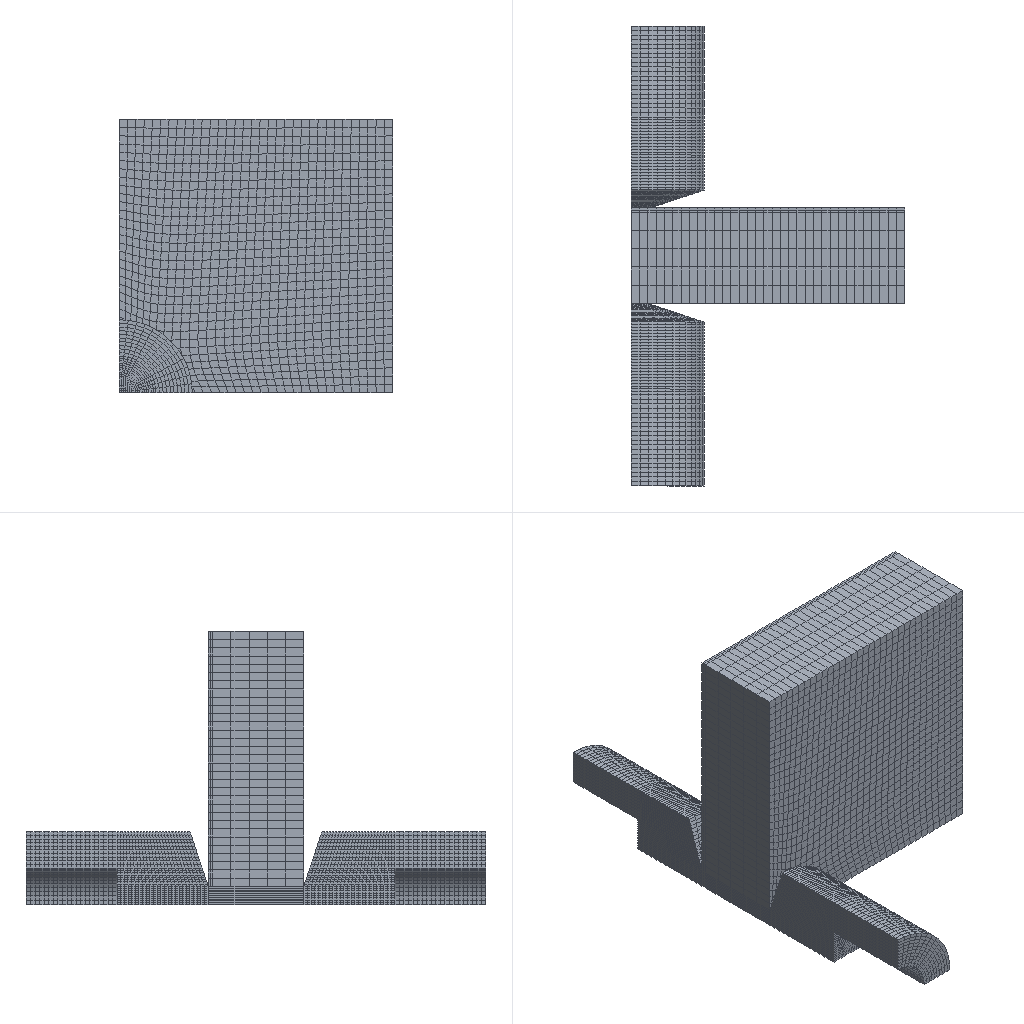Simulation study | abaqus
Set-up summary:
category,name,step,type,value,unit,region
solver,abaqus
solver,version,,,Abaqus/Standard 2020
units,not stated in the deck,,not stated
analysis,deck,,coupled temperature-displacement,coupled temperature-displacement
load_step,Step-1,Step-1,coupled temperature-displacement,nlgeom=True
contact,interactions,,,general=1 pairs=3 ties=0
load_step,requested,,,1
mesh,nodes,,,35020
mesh,elements,,,28627
element_type,Q3D8R,,solid,28627
load,load commands in deck,,count,2
bc,support commands in deck,,count,7
material,SUS301,,in results
material,TDJ,,in results
check,setup vs results,,match,"per instance, exact: element labels, types and connectivity; labels of the nodes the elements use; coordinates of those nodes at SINGLE_PRECISION in 3 of 4 instance(s)"
Abaqus input file, long lists of numbers shortened:
*Heading
** Job name: Job-2 Model name: djdh
** Generated by: Abaqus/CAE 2020
*Preprint, echo=NO, model=NO, history=NO, contact=NO
**
** PARTS
**
*Part, name=BAN1
*Node
      1,           0.,           2.,           0.
      2,           0.,           2.,          0.5
** (3826 more lines like these left out)
*Element, type=Q3D8R
   1,  372,  373, 2781, 2724,   38,   39,  330,  329
   2,  373,  374, 2782, 2781,   39,   40,  331,  330
** (2400 more lines like these left out)
*Nset, nset=SET-1, generate
    1,  3828,     1
*Elset, elset=SET-1, generate
    1,  2402,     1
*Nset, nset=_PICKEDSET159, internal, generate
    1,  3828,     1
*Elset, elset=_PICKEDSET159, internal, generate
    1,  2402,     1
** Section: Section-1-_PICKEDSET159
*Solid Section, elset=_PICKEDSET159, material=SUS301
,
*End Part
**
*Part, name=BAN2
*Node
      1,           0.,           2.,           0.
      2,           0.,           2.,          10.
** (7558 more lines like these left out)
*Element, type=Q3D8R
   1,  507,  508, 4387, 3229,   39,   40,  344,  343
   2,  508,  509, 4388, 4387,   40,   41,  345,  344
** (5923 more lines like these left out)
*Nset, nset=SET-1, generate
    1,  7560,     1
*Elset, elset=SET-1, generate
    1,  5925,     1
*Nset, nset=_PICKEDSET107, internal, generate
    1,  7560,     1
*Elset, elset=_PICKEDSET107, internal, generate
    1,  5925,     1
** Section: Section-2-_PICKEDSET107
*Solid Section, elset=_PICKEDSET107, material=SUS301
,
*End Part
**
*Part, name=SDJ
*Node
      1,           0.,           0.,           2.
      2,           0.,           0.,           0.
** (11814 more lines like these left out)
*Element, type=Q3D8R
    1,   717,   718,  4214,  3902,    25,    26,   472,   471
    2,   718,   719,  4215,  4214,    26,    27,   473,   472
** (10148 more lines like these left out)
*Nset, nset=SET-1, generate
     1,  11816,      1
*Elset, elset=SET-1, generate
     1,  10150,      1
** Section: Section-3-SET-1
*Solid Section, elset=SET-1, material=TDJ
,
*End Part
**
*Part, name=XDJ
*Node
      1,           8.,  -11.6,           0.
      2,           0.,  -11.6,           8.
** (11814 more lines like these left out)
*Element, type=Q3D8R
    1,   160,  1269,  3861,   927,     1,    19,   471,    80
    2,  1269,  1270,  3862,  3861,    19,    20,   472,   471
** (10148 more lines like these left out)
*Nset, nset=SET-1, generate
     1,  11816,      1
*Elset, elset=SET-1, generate
     1,  10150,      1
** Section: Section-4-SET-1
*Solid Section, elset=SET-1, material=TDJ
,
*End Part
**
**
** ASSEMBLY
**
*Assembly, name=Assembly
**
*Instance, name=BAN1-1, part=BAN1
          0.,           0.,           0.
          0.,           0.,           0., 1.,           0.,           0., 90.
*End Instance
**
*Instance, name=BAN2-1, part=BAN2
          0.,         -0.5,           0.
          0.,         -0.5,           0., 1.,         -0.5,           0., 90.
*End Instance
**
*Instance, name=SDJ-1, part=SDJ
*End Instance
**
*Instance, name=XDJ-1, part=XDJ
          0.,         -8.9,           0.
*End Instance
**
*Node
      1,           0.,          20.,    7.6
*Node
      2,           0.,         -30.,           4.
*Nset, nset=SET-1, instance=XDJ-1
    2,    3,    5,    6,    9,   12,   14,   15,   16,   17,   31,   32,   33,   34,   35,   36
   37,   38,   39,   40,   41,   42,   43,   44,   45,   46,   47,   48,   49,   93,   94,   95
** (56 more lines like these left out)
*Nset, nset=SET-1, instance=SDJ-1
    1,    2,    4,    5,   11,   12,   13,   14,   15,   17,   31,   32,   33,   34,   35,   36
   37,   38,   39,   40,   41,   42,   43,   44,   45,   46,   47,   48,   49,   50,   51,   52
** (58 more lines like these left out)
*Elset, elset=SET-1, instance=XDJ-1
    13,    26,    39,    52,    65,    78,    91,   104,   117,   130,   143,   156,   169,   182,   195,   208
   221,   234,   247,   260,   273,   286,   299,   312,   325,   338,   351,   364,   377,   390,   403,   416
** (52 more lines like these left out)
*Elset, elset=SET-1, instance=SDJ-1
    6,   12,   18,   24,   30,   36,   42,   48,   54,   60,   66,   72,   78,   84,   90,   96
  102,  108,  114,  120,  126,  132,  138,  144,  145,  146,  147,  148,  149,  150,  151,  187
** (53 more lines like these left out)
*Nset, nset=SET-2, instance=XDJ-1
    2,    3,    5,    6,    9,   12,   14,   15,   16,   17,   31,   32,   33,   34,   35,   36
   37,   38,   39,   40,   41,   42,   43,   44,   45,   46,   47,   48,   49,   93,   94,   95
** (56 more lines like these left out)
*Nset, nset=SET-2, instance=SDJ-1
    1,    2,    4,    5,   11,   12,   13,   14,   15,   17,   31,   32,   33,   34,   35,   36
   37,   38,   39,   40,   41,   42,   43,   44,   45,   46,   47,   48,   49,   50,   51,   52
** (58 more lines like these left out)
*Elset, elset=SET-2, instance=XDJ-1
    13,    26,    39,    52,    65,    78,    91,   104,   117,   130,   143,   156,   169,   182,   195,   208
   221,   234,   247,   260,   273,   286,   299,   312,   325,   338,   351,   364,   377,   390,   403,   416
** (52 more lines like these left out)
*Elset, elset=SET-2, instance=SDJ-1
    6,   12,   18,   24,   30,   36,   42,   48,   54,   60,   66,   72,   78,   84,   90,   96
  102,  108,  114,  120,  126,  132,  138,  144,  145,  146,  147,  148,  149,  150,  151,  187
** (53 more lines like these left out)
*Nset, nset=SET-3, instance=XDJ-1
    1,    4,    7,    8,   10,   11,   13,   15,   16,   18,   62,   63,   64,   65,   66,   67
   68,   69,   70,   71,   72,   73,   74,   75,   76,   77,   78,   79,   80,  124,  125,  126
** (58 more lines like these left out)
*Nset, nset=SET-3, instance=SDJ-1
    2,    3,    5,    6,    7,    8,    9,   10,   16,   18,   63,   64,   65,   66,   67,   68
   69,   70,   71,   72,   73,   74,   75,   76,   77,   78,   79,   80,   81,   82,   83,   84
** (56 more lines like these left out)
*Elset, elset=SET-3, instance=XDJ-1
     1,    14,    27,    40,    53,    66,    79,    92,   105,   118,   131,   144,   157,   170,   183,   196
   209,   222,   235,   248,   261,   274,   287,   300,   313,   326,   339,   352,   365,   378,   391,   404
** (53 more lines like these left out)
*Elset, elset=SET-3, instance=SDJ-1
   151,   158,   165,   172,   179,   186,   193,   200,   207,   214,   221,   228,   235,   242,   249,   256
   263,   270,   277,   284,   291,   298,   305,   312,   319,   326,   333,   340,   347,   354,   361,   368
** (52 more lines like these left out)
*Nset, nset=SET-4, instance=XDJ-1
    3,    4,    6,    7,   50,   51,   52,   53,   54,   55,   56,   57,   58,   59,   60,   61
  112,  113,  114,  115,  116,  117,  118,  119,  120,  121,  122,  123,  143,  144,  145,  146
** (8 more lines like these left out)
*Elset, elset=SET-4, instance=XDJ-1
  248,  249,  250,  251,  252,  253,  254,  255,  256,  257,  258,  259,  260,  508,  509,  510
  511,  512,  513,  514,  515,  516,  517,  518,  519,  520,  768,  769,  770,  771,  772,  773
** (7 more lines like these left out)
*Nset, nset=SET-5, instance=XDJ-1
    3,    4,    6,    7,   50,   51,   52,   53,   54,   55,   56,   57,   58,   59,   60,   61
  112,  113,  114,  115,  116,  117,  118,  119,  120,  121,  122,  123,  143,  144,  145,  146
** (8 more lines like these left out)
*Elset, elset=SET-5, instance=XDJ-1
  248,  249,  250,  251,  252,  253,  254,  255,  256,  257,  258,  259,  260,  508,  509,  510
  511,  512,  513,  514,  515,  516,  517,  518,  519,  520,  768,  769,  770,  771,  772,  773
** (7 more lines like these left out)
*Nset, nset=SET-6, instance=SDJ-1
   15,   16,   17,   18,  372,  373,  374,  375,  376,  377,  378,  379,  380,  381,  382,  383
  422,  423,  424,  425,  426,  427,  428,  429,  430,  431,  432,  433,  453,  454,  455,  456
** (8 more lines like these left out)
*Elset, elset=SET-6, instance=SDJ-1, generate
  7570,  10150,     20
*Nset, nset=SET-7, instance=BAN1-1
    3,    4,    7,    8,    9,   10,   11,   12,  100,  101,  102,  103,  104,  105,  106,  107
  108,  109,  110,  111,  112,  113,  114,  115,  116,  117,  118,  119,  120,  121,  122,  123
** (11 more lines like these left out)
*Nset, nset=SET-7, instance=BAN2-1
    3,    4,    7,    8,    9,   10,   11,   12,   99,  100,  101,  102,  103,  104,  105,  106
  107,  108,  109,  110,  111,  112,  113,  114,  115,  116,  117,  118,  119,  120,  121,  122
** (24 more lines like these left out)
*Nset, nset=SET-7, instance=SDJ-1, generate
     1,  11816,      1
*Nset, nset=SET-7, instance=XDJ-1, generate
     1,  11816,      1
*Elset, elset=SET-7, instance=BAN1-1
   96,  122,  148,  174,  200,  226,  252,  253,  279,  305,  331,  357,  383,  409,  505,  506
  507,  508,  509,  510,  511,  512,  513,  514,  515,  516,  517,  518,  519,  520,  521,  522
** (7 more lines like these left out)
*Elset, elset=SET-7, instance=BAN2-1
  147,  174,  201,  228,  255,  282,  309,  336,  363,  390,  417,  444,  471,  498,  525,  552
  579,  606,  607,  608,  661,  662,  715,  716,  769,  770,  823,  824,  877,  878, 1051, 1052
** (19 more lines like these left out)
*Elset, elset=SET-7, instance=SDJ-1, generate
     1,  10150,      1
*Elset, elset=SET-7, instance=XDJ-1, generate
     1,  10150,      1
*Nset, nset=SET-11, instance=XDJ-1
    2,    3,    5,    6,    9,   12,   14,   15,   16,   17,   31,   32,   33,   34,   35,   36
   37,   38,   39,   40,   41,   42,   43,   44,   45,   46,   47,   48,   49,   93,   94,   95
** (56 more lines like these left out)
*Nset, nset=SET-11, instance=SDJ-1
    1,    2,    4,    5,   11,   12,   13,   14,   15,   17,   31,   32,   33,   34,   35,   36
   37,   38,   39,   40,   41,   42,   43,   44,   45,   46,   47,   48,   49,   50,   51,   52
** (58 more lines like these left out)
*Elset, elset=SET-11, instance=XDJ-1
    13,    26,    39,    52,    65,    78,    91,   104,   117,   130,   143,   156,   169,   182,   195,   208
   221,   234,   247,   260,   273,   286,   299,   312,   325,   338,   351,   364,   377,   390,   403,   416
** (52 more lines like these left out)
*Elset, elset=SET-11, instance=SDJ-1
    6,   12,   18,   24,   30,   36,   42,   48,   54,   60,   66,   72,   78,   84,   90,   96
  102,  108,  114,  120,  126,  132,  138,  144,  145,  146,  147,  148,  149,  150,  151,  187
** (53 more lines like these left out)
*Nset, nset=SET-12, instance=XDJ-1
    1,    4,    7,    8,   10,   11,   13,   15,   16,   18,   62,   63,   64,   65,   66,   67
   68,   69,   70,   71,   72,   73,   74,   75,   76,   77,   78,   79,   80,  124,  125,  126
** (58 more lines like these left out)
*Nset, nset=SET-12, instance=SDJ-1
    2,    3,    5,    6,    7,    8,    9,   10,   16,   18,   63,   64,   65,   66,   67,   68
   69,   70,   71,   72,   73,   74,   75,   76,   77,   78,   79,   80,   81,   82,   83,   84
** (56 more lines like these left out)
*Elset, elset=SET-12, instance=XDJ-1
     1,    14,    27,    40,    53,    66,    79,    92,   105,   118,   131,   144,   157,   170,   183,   196
   209,   222,   235,   248,   261,   274,   287,   300,   313,   326,   339,   352,   365,   378,   391,   404
** (53 more lines like these left out)
*Elset, elset=SET-12, instance=SDJ-1
   151,   158,   165,   172,   179,   186,   193,   200,   207,   214,   221,   228,   235,   242,   249,   256
   263,   270,   277,   284,   291,   298,   305,   312,   319,   326,   333,   340,   347,   354,   361,   368
** (52 more lines like these left out)
*Nset, nset=Set-49, instance=XDJ-1
    3,    4,    6,    7,   50,   51,   52,   53,   54,   55,   56,   57,   58,   59,   60,   61
  112,  113,  114,  115,  116,  117,  118,  119,  120,  121,  122,  123,  143,  144,  145,  146
** (8 more lines like these left out)
*Nset, nset=Set-50, instance=SDJ-1
   15,   16,   17,   18,  372,  373,  374,  375,  376,  377,  378,  379,  380,  381,  382,  383
  422,  423,  424,  425,  426,  427,  428,  429,  430,  431,  432,  433,  453,  454,  455,  456
** (8 more lines like these left out)
*Nset, nset=Set-51, instance=XDJ-1
    5,    8,   13,   14,   15,   81,   82,   83,   84,   85,   86,   87,   88,   89,   90,   91
   92,  217,  218,  219,  220,  221,  222,  223,  224,  225,  226,  227,  228,  229,  230,  231
** (11 more lines like these left out)
*Nset, nset=Set-56, instance=BAN2-1
    2,    3,    6,    9,   10,   12,   58,   59,   60,   61,   62,   63,   64,   65,   66,   67
   68,   69,   70,   71,   72,   73,   74,   75,   76,   77,   78,   79,   80,   81,   82,   83
** (77 more lines like these left out)
*Nset, nset=Set-57, instance=BAN1-1
    1,    5,   11,   44,   45,   46,   47,   48,   49,   50,   51,   52,   53,   54,   55,   56
  292,  293,  294,  295,  296,  297,  298,  299,  300,  301,  302,  303,  304,  305,  306,  307
** (5 more lines like these left out)
*Nset, nset=Set-58, instance=BAN1-1
    1,    5,   11,   27,   28,   29,   30,   31,   32,   33,   34,   35,   36,   37,   38,   39
   40,   41,   42,   44,   45,   46,   47,   48,   49,   50,   51,   52,   53,   54,   55,   56
** (31 more lines like these left out)
*Nset, nset=Set-59, instance=SDJ-1
    4,    5,    6,    8,   11,  118,  119,  120,  121,  122,  123,  124,  125,  126,  127,  128
  129,  130,  131,  132,  133,  134,  135,  136,  137,  138,  139,  140,  141,  142,  143,  144
** (11 more lines like these left out)
*Nset, nset=Set-60, instance=XDJ-1
    3,    4,    6,    7,   50,   51,   52,   53,   54,   55,   56,   57,   58,   59,   60,   61
  112,  113,  114,  115,  116,  117,  118,  119,  120,  121,  122,  123,  143,  144,  145,  146
** (8 more lines like these left out)
*Nset, nset=Set-61, instance=XDJ-1
    5,    8,   13,   14,   15,   81,   82,   83,   84,   85,   86,   87,   88,   89,   90,   91
   92,  217,  218,  219,  220,  221,  222,  223,  224,  225,  226,  227,  228,  229,  230,  231
** (11 more lines like these left out)
*Nset, nset=Set-62, instance=SDJ-1
   15,   16,   17,   18,  372,  373,  374,  375,  376,  377,  378,  379,  380,  381,  382,  383
  422,  423,  424,  425,  426,  427,  428,  429,  430,  431,  432,  433,  453,  454,  455,  456
** (8 more lines like these left out)
*Nset, nset=Set-63, instance=BAN2-1
    2,    3,    6,    9,   10,   12,   58,   59,   60,   61,   62,   63,   64,   65,   66,   67
   68,   69,   70,   71,   72,   73,   74,   75,   76,   77,   78,   79,   80,   81,   82,   83
** (77 more lines like these left out)
*Nset, nset=Set-64, instance=BAN2-1
    2,    3,    6,    9,   10,   12,   58,   59,   60,   61,   62,   63,   64,   65,   66,   67
   68,   69,   70,   71,   72,   73,   74,   75,   76,   77,   78,   79,   80,   81,   82,   83
** (77 more lines like these left out)
*Nset, nset=Set-65, instance=BAN1-1
    1,    4,    5,    7,    8,   11,   13,   14,   15,   16,   17,   18,   19,   20,   21,   22
   23,   24,   25,   26,   27,   28,   29,   30,   31,   32,   33,   34,   35,   36,   37,   38
** (78 more lines like these left out)
*Nset, nset=Set-66, instance=SDJ-1
    4,    5,    6,    8,   11,  118,  119,  120,  121,  122,  123,  124,  125,  126,  127,  128
  129,  130,  131,  132,  133,  134,  135,  136,  137,  138,  139,  140,  141,  142,  143,  144
** (11 more lines like these left out)
*Nset, nset=Set-67, instance=XDJ-1
    3,    4,    6,    7,   50,   51,   52,   53,   54,   55,   56,   57,   58,   59,   60,   61
  112,  113,  114,  115,  116,  117,  118,  119,  120,  121,  122,  123,  143,  144,  145,  146
** (8 more lines like these left out)
*Nset, nset=Set-68, instance=SDJ-1
   15,   16,   17,   18,  372,  373,  374,  375,  376,  377,  378,  379,  380,  381,  382,  383
  422,  423,  424,  425,  426,  427,  428,  429,  430,  431,  432,  433,  453,  454,  455,  456
** (8 more lines like these left out)
*Elset, elset=b_Set-52, instance=SDJ-1, generate
     1,  10150,      1
*Elset, elset=b_Set-54, instance=XDJ-1, generate
     1,  10150,      1
*Elset, elset=_M_SURF-1_S2, internal, instance=SDJ-1
   1,   2,   3,   4,   5,   6,   7,   8,   9,  10,  11,  12, 145, 146, 147, 148
 149, 150, 151, 152, 153, 154, 155, 156, 157, 158, 159, 160, 161, 162, 163, 164
** (3 more lines like these left out)
*Elset, elset=_M_SURF-3_S3, internal, instance=XDJ-1
 6173, 6174, 6175, 6176, 6177, 6178, 6179, 6264, 6265, 6266, 6267, 6268, 6269, 6270
*Elset, elset=_M_SURF-3_S4, internal, instance=XDJ-1
 6029, 6042, 6055, 6068, 6081, 6094, 6107, 6120, 6133, 6146, 6159, 6172, 6367, 6380, 6393, 6406
 6419, 6432, 6445, 6458, 6471, 6484, 6497, 6510, 6523, 6536, 6549, 6562, 6575, 6588, 6601, 6614
** (2 more lines like these left out)
*Nset, nset=_PICKEDSET39, internal, instance=XDJ-1
    3,    4,    6,    7,   50,   51,   52,   53,   54,   55,   56,   57,   58,   59,   60,   61
  112,  113,  114,  115,  116,  117,  118,  119,  120,  121,  122,  123,  143,  144,  145,  146
** (8 more lines like these left out)
*Elset, elset=_PICKEDSET39, internal, instance=XDJ-1
  248,  249,  250,  251,  252,  253,  254,  255,  256,  257,  258,  259,  260,  508,  509,  510
  511,  512,  513,  514,  515,  516,  517,  518,  519,  520,  768,  769,  770,  771,  772,  773
** (7 more lines like these left out)
*Nset, nset=_PICKEDSET41, internal, instance=XDJ-1
    3,    4,    6,    7,   50,   51,   52,   53,   54,   55,   56,   57,   58,   59,   60,   61
  112,  113,  114,  115,  116,  117,  118,  119,  120,  121,  122,  123,  143,  144,  145,  146
** (8 more lines like these left out)
*Elset, elset=_PICKEDSET41, internal, instance=XDJ-1
  248,  249,  250,  251,  252,  253,  254,  255,  256,  257,  258,  259,  260,  508,  509,  510
  511,  512,  513,  514,  515,  516,  517,  518,  519,  520,  768,  769,  770,  771,  772,  773
** (7 more lines like these left out)
*Nset, nset=_PICKEDSET57, internal, instance=BAN1-1, generate
    1,  3828,     1
*Nset, nset=_PICKEDSET57, internal, instance=BAN2-1, generate
    1,  7560,     1
*Nset, nset=_PICKEDSET57, internal, instance=SDJ-1, generate
     1,  11816,      1
*Nset, nset=_PICKEDSET57, internal, instance=XDJ-1, generate
     1,  11816,      1
*Elset, elset=_PICKEDSET57, internal, instance=BAN1-1, generate
    1,  2402,     1
*Elset, elset=_PICKEDSET57, internal, instance=BAN2-1, generate
    1,  5925,     1
*Elset, elset=_PICKEDSET57, internal, instance=SDJ-1, generate
     1,  10150,      1
*Elset, elset=_PICKEDSET57, internal, instance=XDJ-1, generate
     1,  10150,      1
*Nset, nset=_PICKEDSET73, internal, instance=BAN1-1
    1,    2,    3,    4,   11,   12,   13,   14,   15,   16,   17,   18,   19,   20,   21,   22
   23,   24,   25,   26,   27,   28,   29,   30,   31,   32,   33,   34,   35,   36,   37,   38
** (6 more lines like these left out)
*Nset, nset=_PICKEDSET73, internal, instance=BAN2-1
    1,    2,    3,    4,   11,   12,   13,   14,   15,   16,   17,   18,   19,   20,   21,   22
   23,   24,   25,   26,   27,   28,   29,   30,   31,   32,   33,   34,   35,   36,   37,   38
** (14 more lines like these left out)
*Nset, nset=_PICKEDSET73, internal, instance=SDJ-1
    1,    2,    4,    5,   11,   12,   13,   14,   15,   17,   31,   32,   33,   34,   35,   36
   37,   38,   39,   40,   41,   42,   43,   44,   45,   46,   47,   48,   49,   50,   51,   52
** (58 more lines like these left out)
*Nset, nset=_PICKEDSET73, internal, instance=XDJ-1
    2,    3,    5,    6,    9,   12,   14,   15,   16,   17,   31,   32,   33,   34,   35,   36
   37,   38,   39,   40,   41,   42,   43,   44,   45,   46,   47,   48,   49,   93,   94,   95
** (56 more lines like these left out)
*Elset, elset=_PICKEDSET73, internal, instance=BAN1-1
    1,    2,    3,    4,    5,   36,   37,   38,   39,   40,   71,   72,   73,   74,   75,   76
   77,   78,   79,   80,   81,   82,   83,   84,   85,   86,   87,   88,   89,   90,   91,   92
** (4 more lines like these left out)
*Elset, elset=_PICKEDSET73, internal, instance=BAN2-1
    1,    2,    3,    4,    5,    6,    7,    8,   49,   50,   51,   52,   53,   54,   55,   56
   57,   58,   59,   60,  121,  122,  123,  124,  125,  126,  127,  128,  129,  130,  131,  132
** (11 more lines like these left out)
*Elset, elset=_PICKEDSET73, internal, instance=SDJ-1
    6,   12,   18,   24,   30,   36,   42,   48,   54,   60,   66,   72,   78,   84,   90,   96
  102,  108,  114,  120,  126,  132,  138,  144,  145,  146,  147,  148,  149,  150,  151,  187
** (53 more lines like these left out)
*Elset, elset=_PICKEDSET73, internal, instance=XDJ-1
    13,    26,    39,    52,    65,    78,    91,   104,   117,   130,   143,   156,   169,   182,   195,   208
   221,   234,   247,   260,   273,   286,   299,   312,   325,   338,   351,   364,   377,   390,   403,   416
** (52 more lines like these left out)
*Nset, nset=_PICKEDSET74, internal, instance=BAN1-1
    5,    6,    8,   10,   11,   12,  165,  166,  167,  168,  169,  170,  171,  172,  173,  174
  175,  176,  177,  178,  179,  180,  181,  182,  183,  184,  185,  186,  187,  188,  189,  190
** (6 more lines like these left out)
*Nset, nset=_PICKEDSET74, internal, instance=BAN2-1
    5,    6,    8,   10,   11,   12,  167,  168,  169,  170,  171,  172,  173,  174,  175,  176
  177,  178,  179,  180,  181,  182,  183,  184,  185,  186,  187,  188,  189,  190,  191,  192
** (14 more lines like these left out)
*Nset, nset=_PICKEDSET74, internal, instance=SDJ-1
    2,    3,    5,    6,    7,    8,    9,   10,   16,   18,   63,   64,   65,   66,   67,   68
   69,   70,   71,   72,   73,   74,   75,   76,   77,   78,   79,   80,   81,   82,   83,   84
** (56 more lines like these left out)
*Nset, nset=_PICKEDSET74, internal, instance=XDJ-1
    1,    4,    7,    8,   10,   11,   13,   15,   16,   18,   62,   63,   64,   65,   66,   67
   68,   69,   70,   71,   72,   73,   74,   75,   76,   77,   78,   79,   80,  124,  125,  126
** (58 more lines like these left out)
*Elset, elset=_PICKEDSET74, internal, instance=BAN1-1
  441,  448,  455,  462,  469,  470,  477,  484,  491,  498, 1187, 1194, 1201, 1208, 1215, 1222
 1229, 1236, 1243, 1250, 1257, 1264, 1271, 1278, 1285, 1292, 1299, 1306, 1313, 1320, 1327, 1334
** (4 more lines like these left out)
*Elset, elset=_PICKEDSET74, internal, instance=BAN2-1
  936,  942,  948,  954,  960,  966,  972,  978,  979,  980,  981,  997,  998,  999, 1015, 1016
 1017, 1033, 1034, 1035, 2514, 2520, 2526, 2532, 2538, 2544, 2550, 2556, 2562, 2568, 2574, 2580
** (11 more lines like these left out)
*Elset, elset=_PICKEDSET74, internal, instance=SDJ-1
   151,   158,   165,   172,   179,   186,   193,   200,   207,   214,   221,   228,   235,   242,   249,   256
   263,   270,   277,   284,   291,   298,   305,   312,   319,   326,   333,   340,   347,   354,   361,   368
** (52 more lines like these left out)
*Elset, elset=_PICKEDSET74, internal, instance=XDJ-1
     1,    14,    27,    40,    53,    66,    79,    92,   105,   118,   131,   144,   157,   170,   183,   196
   209,   222,   235,   248,   261,   274,   287,   300,   313,   326,   339,   352,   365,   378,   391,   404
** (53 more lines like these left out)
*Nset, nset=_PICKEDSET80, internal, instance=SDJ-1
   15,   16,   17,   18,  372,  373,  374,  375,  376,  377,  378,  379,  380,  381,  382,  383
  422,  423,  424,  425,  426,  427,  428,  429,  430,  431,  432,  433,  453,  454,  455,  456
** (8 more lines like these left out)
*Elset, elset=_PICKEDSET80, internal, instance=SDJ-1, generate
  7570,  10150,     20
*Nset, nset=_PICKEDSET81, internal, instance=SDJ-1
   15,   16,   17,   18,  372,  373,  374,  375,  376,  377,  378,  379,  380,  381,  382,  383
  422,  423,  424,  425,  426,  427,  428,  429,  430,  431,  432,  433,  453,  454,  455,  456
** (8 more lines like these left out)
*Elset, elset=_PICKEDSET81, internal, instance=SDJ-1, generate
  7570,  10150,     20
*Nset, nset=_PickedSet141, internal
 1,
*Nset, nset=_PickedSet143, internal
 2,
*Elset, elset=_SURF-7_S2, internal, instance=SDJ-1, generate
 7551,  7810,     1
*Elset, elset=_SURF-8_S1, internal, instance=XDJ-1, generate
 2341,  2600,     1
*Elset, elset=_SURF-9_S4, internal, instance=SDJ-1, generate
  7570,  10150,     20
*Elset, elset=_SURF-10_S4, internal, instance=SDJ-1, generate
  7570,  10150,     20
*Elset, elset=_SURF-14_S1, internal, instance=SDJ-1, generate
 7447,  7550,     1
*Elset, elset=_SURF-14_S1, internal, instance=XDJ-1
 2341, 2342, 2343, 2344, 2345, 2346, 2347, 2348, 2349, 2350, 2351, 2352, 2353, 2354, 2355, 2356
 2357, 2358, 2359, 2360, 2361, 2362, 2363, 2364, 2365, 2366, 2367, 2368, 2369, 2370, 2371, 2372
** (21 more lines like these left out)
*Elset, elset=_SURF-14_S2, internal, instance=SDJ-1, generate
 7551,  7810,     1
*Elset, elset=_SURF-14_S2, internal, instance=XDJ-1
 5201, 5202, 5203, 5204, 5205, 5206, 5207, 5208, 5209, 5210, 5211, 5212, 5345, 5346, 5347, 5348
 5349, 5350, 5351, 5352, 5353, 5354, 5355, 5356, 5357, 5358, 5513, 5514, 5515, 5516, 5517, 5518
** (3 more lines like these left out)
*Elset, elset=_SURF-14_S3, internal, instance=SDJ-1
  973,  974,  975,  976,  977,  978,  979, 1064, 1065, 1066, 1067, 1068, 1069, 1070, 1155, 1156
 1157, 1158, 1159, 1160, 1161, 1246, 1247, 1248, 1249, 1250, 1251, 1252, 1337, 1338, 1339, 1340
** (1 more lines like these left out)
*Elset, elset=_SURF-14_S4, internal, instance=SDJ-1
  829,  842,  855,  868,  881,  894,  907,  920,  933,  946,  959,  972, 1531, 1544, 1557, 1570
 1583, 1596, 1609, 1622, 1635, 1648, 1661, 1674, 1687, 1700
*Elset, elset=__PICKEDSURF42_S4, internal, instance=SDJ-1, generate
  7570,  10150,     20
*Elset, elset=__PICKEDSURF59_S1, internal, instance=SDJ-1, generate
  9891,  10150,      1
*Elset, elset=__PICKEDSURF59_S2, internal, instance=BAN1-1, generate
  505,  1388,     1
*Elset, elset=__PICKEDSURF59_S2, internal, instance=BAN2-1
 2833, 2834, 2835, 2836, 2837, 2838, 2839, 2840, 2841, 2842, 2843, 2844, 2845, 2846, 2847, 2848
 2849, 2850, 2851, 2852, 2853, 2854, 2855, 2856, 2857, 2858, 2859, 2860, 2861, 2862, 2863, 2864
** (14 more lines like these left out)
*Elset, elset=__PICKEDSURF59_S2, internal, instance=SDJ-1, generate
 4951,  5054,     1
*Elset, elset=__PICKEDSURF59_S2, internal, instance=XDJ-1
    1,    2,    3,    4,    5,    6,    7,    8,    9,   10,   11,   12,   13,   14,   15,   16
   17,   18,   19,   20,   21,   22,   23,   24,   25,   26,   27,   28,   29,   30,   31,   32
** (29 more lines like these left out)
*Elset, elset=__PICKEDSURF59_S3, internal, instance=BAN1-1
    1,    2,    3,    4,    5,    6,    7,    8,    9,   10,   11,   12,   13,   14,   15,   16
   17,   18,   19,   20,   21,   22,   23,   24,   25,   26,   27,   28,   29,   30,   31,   32
** (5 more lines like these left out)
*Elset, elset=__PICKEDSURF59_S3, internal, instance=BAN2-1
  121,  122,  123,  124,  125,  126,  127,  128,  129,  130,  131,  132,  133,  134,  135,  136
  137,  138,  139,  140,  141,  142,  143,  144,  145,  146,  147,  202,  203,  204,  205,  206
** (59 more lines like these left out)
*Elset, elset=__PICKEDSURF59_S4, internal, instance=BAN1-1
   96,  122,  148,  174,  200,  226,  252,  253,  254,  255,  256,  257,  258,  259,  260,  261
  262,  263,  264,  265,  266,  267,  268,  269,  270,  271,  272,  273,  274,  275,  276,  277
** (14 more lines like these left out)
*Elset, elset=__PICKEDSURF59_S4, internal, instance=BAN2-1
   51,   54,   57,   60,   63,   66,   69,   72,   75,   78,   81,   84,   87,   90,   93,   96
   99,  102,  105,  108,  111,  114,  117,  120,  147,  174,  201,  228,  255,  282,  309,  336
** (12 more lines like these left out)
*Elset, elset=__PICKEDSURF59_S5, internal, instance=XDJ-1
  7018,  7019,  7020,  7021,  7022,  7023,  7024,  7025,  7026,  7027,  7028,  7029,  7030,  7148,  7149,  7150
  7151,  7152,  7153,  7154,  7155,  7156,  7157,  7158,  7159,  7160,  7278,  7279,  7280,  7281,  7282,  7283
** (19 more lines like these left out)
*Elset, elset=__PICKEDSURF59_S5, internal, instance=SDJ-1
 1926, 1927, 1928, 1929, 1930, 1931, 1932, 1933, 1934, 1935, 1936, 1937, 1938, 1939, 1940, 1941
 1942, 1943, 1944, 1945, 1946, 1947, 1948, 1949, 1950, 2176, 2177, 2178, 2179, 2180, 2181, 2182
** (19 more lines like these left out)
*Elset, elset=__PICKEDSURF59_S6, internal, instance=SDJ-1, generate
 1701,  4926,    25
*Elset, elset=__PICKEDSURF60_S2, internal, instance=SDJ-1
   1,   2,   3,   4,   5,   6,   7,   8,   9,  10,  11,  12, 145, 146, 147, 148
 149, 150, 151, 152, 153, 154, 155, 156, 157, 158, 159, 160, 161, 162, 163, 164
** (3 more lines like these left out)
*Elset, elset=__PICKEDSURF61_S2, internal, instance=BAN1-1, generate
 2221,  2311,     1
*Elset, elset=__PICKEDSURF62_S3, internal, instance=XDJ-1
 6173, 6174, 6175, 6176, 6177, 6178, 6179, 6264, 6265, 6266, 6267, 6268, 6269, 6270
*Elset, elset=__PICKEDSURF62_S4, internal, instance=XDJ-1
 6029, 6042, 6055, 6068, 6081, 6094, 6107, 6120, 6133, 6146, 6159, 6172, 6367, 6380, 6393, 6406
 6419, 6432, 6445, 6458, 6471, 6484, 6497, 6510, 6523, 6536, 6549, 6562, 6575, 6588, 6601, 6614
** (2 more lines like these left out)
*Elset, elset=__PICKEDSURF63_S3, internal, instance=BAN2-1
 5674, 5675, 5676, 5677, 5678, 5679, 5692, 5693, 5694, 5695, 5696, 5697, 5710, 5711, 5712, 5713
 5714, 5715, 5728, 5729, 5730, 5731, 5732, 5733, 5818, 5819, 5820, 5821, 5822, 5823, 5836, 5837
** (2 more lines like these left out)
*Elset, elset=__PICKEDSURF63_S4, internal, instance=BAN2-1, generate
 5748,  5817,     3
*Elset, elset=__PICKEDSURF66_S2, internal, instance=BAN1-1, generate
 2039,  2220,     1
*Elset, elset=__PICKEDSURF66_S3, internal, instance=BAN1-1
   71,   72,   73,   74,   75,   76,   77,   78,   79,   80,   81,   82,   83,   84,   85,   86
   87,   88,   89,   90,   91,   92,   93,   94,   95,   96,   97,   98,   99,  100,  101,  102
** (56 more lines like these left out)
*Elset, elset=__PICKEDSURF66_S4, internal, instance=BAN1-1
   36,   37,   38,   39,   40,   41,   42,   43,   44,   45,   46,   47,   48,   49,   50,   51
   52,   53,   54,   55,   56,   57,   58,   59,   60,   61,   62,   63,   64,   65,   66,   67
** (4 more lines like these left out)
*Elset, elset=__PICKEDSURF67_S2, internal, instance=BAN2-1
 1051, 1052, 1053, 1054, 1055, 1056, 1057, 1058, 1059, 1060, 1061, 1062, 1063, 1064, 1065, 1066
 1067, 1068, 1069, 1070, 1071, 1072, 1073, 1074, 1075, 1076, 1077, 1078, 1079, 1080, 1081, 1082
** (59 more lines like these left out)
*Elset, elset=__PICKEDSURF67_S3, internal, instance=BAN2-1
   1,   2,   3,   4,   9,  10,  11,  12,  17,  18,  19,  20,  25,  26,  27,  28
  33,  34,  35,  36,  41,  42,  43,  44, 931, 932, 933, 934, 935, 936, 943, 944
** (1 more lines like these left out)
*Elset, elset=__PICKEDSURF67_S4, internal, instance=BAN2-1, generate
 608,  930,    2
*Elset, elset=__PICKEDSURF82_S4, internal, instance=SDJ-1, generate
  7570,  10150,     20
*Elset, elset=__PICKEDSURF83_S4, internal, instance=SDJ-1, generate
  7570,  10150,     20
*Surface, type=ELEMENT, name=M_SURF-1
_M_SURF-1_S2, S2
*Elset, elset=_M_SURF-3_S4_1, internal, instance=XDJ-1
 6029, 6042, 6055, 6068, 6081, 6094, 6107, 6120, 6133, 6146, 6159, 6172, 6367, 6380, 6393, 6406
 6419, 6432, 6445, 6458, 6471, 6484, 6497, 6510, 6523, 6536, 6549, 6562, 6575, 6588, 6601, 6614
** (2 more lines like these left out)
*Elset, elset=_M_SURF-3_S3_1, internal, instance=XDJ-1
 6173, 6174, 6175, 6176, 6177, 6178, 6179, 6264, 6265, 6266, 6267, 6268, 6269, 6270
*Surface, type=ELEMENT, name=M_SURF-3
_M_SURF-3_S4_1, S4
_M_SURF-3_S3_1, S3
*Surface, type=ELEMENT, name=SURF-7
_SURF-7_S2, S2
*Surface, type=ELEMENT, name=SURF-8
_SURF-8_S1, S1
*Surface, type=ELEMENT, name=SURF-9
_SURF-9_S4, S4
*Surface, type=ELEMENT, name=SURF-10
_SURF-10_S4, S4
*Elset, elset=_SURF-14_S4_1, internal, instance=SDJ-1
  829,  842,  855,  868,  881,  894,  907,  920,  933,  946,  959,  972, 1531, 1544, 1557, 1570
 1583, 1596, 1609, 1622, 1635, 1648, 1661, 1674, 1687, 1700
*Elset, elset=_SURF-14_S3_1, internal, instance=SDJ-1
  973,  974,  975,  976,  977,  978,  979, 1064, 1065, 1066, 1067, 1068, 1069, 1070, 1155, 1156
 1157, 1158, 1159, 1160, 1161, 1246, 1247, 1248, 1249, 1250, 1251, 1252, 1337, 1338, 1339, 1340
** (1 more lines like these left out)
*Elset, elset=_SURF-14_S2_1, internal, instance=SDJ-1, generate
 7551,  7810,     1
*Elset, elset=_SURF-14_S2_1, internal, instance=XDJ-1
 5201, 5202, 5203, 5204, 5205, 5206, 5207, 5208, 5209, 5210, 5211, 5212, 5345, 5346, 5347, 5348
 5349, 5350, 5351, 5352, 5353, 5354, 5355, 5356, 5357, 5358, 5513, 5514, 5515, 5516, 5517, 5518
** (3 more lines like these left out)
*Elset, elset=_SURF-14_S1_1, internal, instance=SDJ-1, generate
 7447,  7550,     1
*Elset, elset=_SURF-14_S1_1, internal, instance=XDJ-1
 2341, 2342, 2343, 2344, 2345, 2346, 2347, 2348, 2349, 2350, 2351, 2352, 2353, 2354, 2355, 2356
 2357, 2358, 2359, 2360, 2361, 2362, 2363, 2364, 2365, 2366, 2367, 2368, 2369, 2370, 2371, 2372
** (21 more lines like these left out)
*Surface, type=ELEMENT, name=SURF-14
_SURF-14_S4_1, S4
_SURF-14_S3_1, S3
_SURF-14_S2_1, S2
_SURF-14_S1_1, S1
*Elset, elset=_Surf-18_S4, internal, instance=SDJ-1, generate
  7570,  10150,     20
*Surface, type=ELEMENT, name=Surf-18
_Surf-18_S4, S4
*Elset, elset=_Surf-19_S1, internal, instance=SDJ-1, generate
 7447,  7550,     1
*Elset, elset=_Surf-19_S3, internal, instance=SDJ-1
  973,  974,  975,  976,  977,  978,  979, 1064, 1065, 1066, 1067, 1068, 1069, 1070, 1155, 1156
 1157, 1158, 1159, 1160, 1161, 1246, 1247, 1248, 1249, 1250, 1251, 1252, 1337, 1338, 1339, 1340
** (1 more lines like these left out)
*Elset, elset=_Surf-19_S4, internal, instance=SDJ-1
  829,  842,  855,  868,  881,  894,  907,  920,  933,  946,  959,  972, 1531, 1544, 1557, 1570
 1583, 1596, 1609, 1622, 1635, 1648, 1661, 1674, 1687, 1700
*Surface, type=ELEMENT, name=Surf-19
_Surf-19_S1, S1
_Surf-19_S3, S3
_Surf-19_S4, S4
*Elset, elset=_Surf-20_S1, internal, instance=XDJ-1, generate
 5097,  5200,     1
*Elset, elset=_Surf-20_S2, internal, instance=XDJ-1
 5201, 5202, 5203, 5204, 5205, 5206, 5207, 5208, 5209, 5210, 5211, 5212, 5345, 5346, 5347, 5348
 5349, 5350, 5351, 5352, 5353, 5354, 5355, 5356, 5357, 5358, 5513, 5514, 5515, 5516, 5517, 5518
** (3 more lines like these left out)
*Surface, type=ELEMENT, name=Surf-20
_Surf-20_S1, S1
_Surf-20_S2, S2
*Elset, elset=_Surf-21_S1, internal, instance=SDJ-1, generate
 7447,  7550,     1
*Elset, elset=_Surf-21_S3, internal, instance=SDJ-1
  973,  974,  975,  976,  977,  978,  979, 1064, 1065, 1066, 1067, 1068, 1069, 1070, 1155, 1156
 1157, 1158, 1159, 1160, 1161, 1246, 1247, 1248, 1249, 1250, 1251, 1252, 1337, 1338, 1339, 1340
** (1 more lines like these left out)
*Elset, elset=_Surf-21_S4, internal, instance=SDJ-1
  829,  842,  855,  868,  881,  894,  907,  920,  933,  946,  959,  972, 1531, 1544, 1557, 1570
 1583, 1596, 1609, 1622, 1635, 1648, 1661, 1674, 1687, 1700
*Surface, type=ELEMENT, name=Surf-21
_Surf-21_S1, S1
_Surf-21_S3, S3
_Surf-21_S4, S4
*Elset, elset=_Surf-26_S4, internal, instance=SDJ-1, generate
  7570,  10150,     20
*Surface, type=ELEMENT, name=Surf-26
_Surf-26_S4, S4
*Elset, elset=_Surf-27_S1, internal, instance=XDJ-1, generate
 5097,  5200,     1
*Elset, elset=_Surf-27_S2, internal, instance=XDJ-1
 5201, 5202, 5203, 5204, 5205, 5206, 5207, 5208, 5209, 5210, 5211, 5212, 5345, 5346, 5347, 5348
 5349, 5350, 5351, 5352, 5353, 5354, 5355, 5356, 5357, 5358, 5513, 5514, 5515, 5516, 5517, 5518
** (3 more lines like these left out)
*Surface, type=ELEMENT, name=Surf-27
_Surf-27_S1, S1
_Surf-27_S2, S2
*Elset, elset=_m_Surf-22_S2, internal, instance=SDJ-1
   1,   2,   3,   4,   5,   6,   7,   8,   9,  10,  11,  12, 145, 146, 147, 148
 149, 150, 151, 152, 153, 154, 155, 156, 157, 158, 159, 160, 161, 162, 163, 164
** (3 more lines like these left out)
*Surface, type=ELEMENT, name=m_Surf-22
_m_Surf-22_S2, S2
*Elset, elset=_m_Surf-24_S3, internal, instance=XDJ-1
 6173, 6174, 6175, 6176, 6177, 6178, 6179, 6264, 6265, 6266, 6267, 6268, 6269, 6270
*Elset, elset=_m_Surf-24_S4, internal, instance=XDJ-1
 6029, 6042, 6055, 6068, 6081, 6094, 6107, 6120, 6133, 6146, 6159, 6172, 6367, 6380, 6393, 6406
 6419, 6432, 6445, 6458, 6471, 6484, 6497, 6510, 6523, 6536, 6549, 6562, 6575, 6588, 6601, 6614
** (2 more lines like these left out)
*Surface, type=ELEMENT, name=m_Surf-24
_m_Surf-24_S3, S3
_m_Surf-24_S4, S4
*Elset, elset=_s_Surf-22_S2, internal, instance=BAN1-1
  505,  506,  507,  508,  509,  510,  511,  512,  513,  514,  515,  516,  517,  518,  519,  520
  521,  522,  523,  524,  525,  526,  527,  528,  529,  530,  531,  532,  533,  534,  535,  536
** (58 more lines like these left out)
*Elset, elset=_s_Surf-22_S3, internal, instance=BAN1-1
   1,   2,   3,   4,   5,   6,   7,   8,   9,  10,  11,  12,  13,  14,  15,  16
  17,  18,  19,  20,  21,  22,  23,  24,  25,  26,  27,  28,  29,  30,  31,  32
** (3 more lines like these left out)
*Elset, elset=_s_Surf-22_S4, internal, instance=BAN1-1, generate
 253,  434,    1
*Surface, type=ELEMENT, name=s_Surf-22
_s_Surf-22_S2, S2
_s_Surf-22_S3, S3
_s_Surf-22_S4, S4
*Elset, elset=_s_Surf-24_S2, internal, instance=BAN2-1, generate
 5020,  5181,     1
*Elset, elset=_s_Surf-24_S3, internal, instance=BAN2-1
  121,  122,  123,  124,  125,  126,  127,  128,  129,  130,  131,  132,  133,  134,  135,  136
  137,  138,  139,  140,  141,  142,  143,  144,  145,  146,  147,  202,  203,  204,  205,  206
** (58 more lines like these left out)
*Elset, elset=_s_Surf-24_S4, internal, instance=BAN2-1
   51,   54,   57,   60,   63,   66,   69,   72,   75,   78,   81,   84,   87,   90,   93,   96
   99,  102,  105,  108,  111,  114,  117,  120,  981,  984,  987,  990,  993,  996,  999, 1002
** (3 more lines like these left out)
*Surface, type=ELEMENT, name=s_Surf-24
_s_Surf-24_S2, S2
_s_Surf-24_S3, S3
_s_Surf-24_S4, S4
*Surface, type=ELEMENT, name=_PICKEDSURF42, internal
__PICKEDSURF42_S4, S4
*Elset, elset=__PICKEDSURF59_S4_1, internal, instance=BAN1-1
   96,  122,  148,  174,  200,  226,  252,  253,  254,  255,  256,  257,  258,  259,  260,  261
  262,  263,  264,  265,  266,  267,  268,  269,  270,  271,  272,  273,  274,  275,  276,  277
** (14 more lines like these left out)
*Elset, elset=__PICKEDSURF59_S4_1, internal, instance=BAN2-1
   51,   54,   57,   60,   63,   66,   69,   72,   75,   78,   81,   84,   87,   90,   93,   96
   99,  102,  105,  108,  111,  114,  117,  120,  147,  174,  201,  228,  255,  282,  309,  336
** (12 more lines like these left out)
*Elset, elset=__PICKEDSURF59_S3_1, internal, instance=BAN1-1
    1,    2,    3,    4,    5,    6,    7,    8,    9,   10,   11,   12,   13,   14,   15,   16
   17,   18,   19,   20,   21,   22,   23,   24,   25,   26,   27,   28,   29,   30,   31,   32
** (5 more lines like these left out)
*Elset, elset=__PICKEDSURF59_S3_1, internal, instance=BAN2-1
  121,  122,  123,  124,  125,  126,  127,  128,  129,  130,  131,  132,  133,  134,  135,  136
  137,  138,  139,  140,  141,  142,  143,  144,  145,  146,  147,  202,  203,  204,  205,  206
** (59 more lines like these left out)
*Elset, elset=__PICKEDSURF59_S2_1, internal, instance=BAN1-1, generate
  505,  1388,     1
*Elset, elset=__PICKEDSURF59_S2_1, internal, instance=BAN2-1
 2833, 2834, 2835, 2836, 2837, 2838, 2839, 2840, 2841, 2842, 2843, 2844, 2845, 2846, 2847, 2848
 2849, 2850, 2851, 2852, 2853, 2854, 2855, 2856, 2857, 2858, 2859, 2860, 2861, 2862, 2863, 2864
** (14 more lines like these left out)
*Elset, elset=__PICKEDSURF59_S2_1, internal, instance=SDJ-1, generate
 4951,  5054,     1
*Elset, elset=__PICKEDSURF59_S2_1, internal, instance=XDJ-1
    1,    2,    3,    4,    5,    6,    7,    8,    9,   10,   11,   12,   13,   14,   15,   16
   17,   18,   19,   20,   21,   22,   23,   24,   25,   26,   27,   28,   29,   30,   31,   32
** (29 more lines like these left out)
*Elset, elset=__PICKEDSURF59_S6_1, internal, instance=SDJ-1, generate
 1701,  4926,    25
*Elset, elset=__PICKEDSURF59_S5_1, internal, instance=SDJ-1
 1926, 1927, 1928, 1929, 1930, 1931, 1932, 1933, 1934, 1935, 1936, 1937, 1938, 1939, 1940, 1941
 1942, 1943, 1944, 1945, 1946, 1947, 1948, 1949, 1950, 2176, 2177, 2178, 2179, 2180, 2181, 2182
** (19 more lines like these left out)
*Elset, elset=__PICKEDSURF59_S5_1, internal, instance=XDJ-1
  7018,  7019,  7020,  7021,  7022,  7023,  7024,  7025,  7026,  7027,  7028,  7029,  7030,  7148,  7149,  7150
  7151,  7152,  7153,  7154,  7155,  7156,  7157,  7158,  7159,  7160,  7278,  7279,  7280,  7281,  7282,  7283
** (19 more lines like these left out)
*Elset, elset=__PICKEDSURF59_S1_1, internal, instance=SDJ-1, generate
  9891,  10150,      1
*Surface, type=ELEMENT, name=_PICKEDSURF59, internal
__PICKEDSURF59_S4_1, S4
__PICKEDSURF59_S3_1, S3
__PICKEDSURF59_S2_1, S2
__PICKEDSURF59_S6_1, S6
__PICKEDSURF59_S5_1, S5
__PICKEDSURF59_S1_1, S1
*Surface, type=ELEMENT, name=_PICKEDSURF60, internal
__PICKEDSURF60_S2, S2
*Surface, type=ELEMENT, name=_PICKEDSURF61, internal
__PICKEDSURF61_S2, S2
*Elset, elset=__PICKEDSURF62_S4_1, internal, instance=XDJ-1
 6029, 6042, 6055, 6068, 6081, 6094, 6107, 6120, 6133, 6146, 6159, 6172, 6367, 6380, 6393, 6406
 6419, 6432, 6445, 6458, 6471, 6484, 6497, 6510, 6523, 6536, 6549, 6562, 6575, 6588, 6601, 6614
** (2 more lines like these left out)
*Elset, elset=__PICKEDSURF62_S3_1, internal, instance=XDJ-1
 6173, 6174, 6175, 6176, 6177, 6178, 6179, 6264, 6265, 6266, 6267, 6268, 6269, 6270
*Surface, type=ELEMENT, name=_PICKEDSURF62, internal
__PICKEDSURF62_S4_1, S4
__PICKEDSURF62_S3_1, S3
*Elset, elset=__PICKEDSURF63_S3_1, internal, instance=BAN2-1
 5674, 5675, 5676, 5677, 5678, 5679, 5692, 5693, 5694, 5695, 5696, 5697, 5710, 5711, 5712, 5713
 5714, 5715, 5728, 5729, 5730, 5731, 5732, 5733, 5818, 5819, 5820, 5821, 5822, 5823, 5836, 5837
** (2 more lines like these left out)
*Elset, elset=__PICKEDSURF63_S4_1, internal, instance=BAN2-1, generate
 5748,  5817,     3
*Surface, type=ELEMENT, name=_PICKEDSURF63, internal
__PICKEDSURF63_S3_1, S3
__PICKEDSURF63_S4_1, S4
*Elset, elset=__PICKEDSURF66_S4_1, internal, instance=BAN1-1
   36,   37,   38,   39,   40,   41,   42,   43,   44,   45,   46,   47,   48,   49,   50,   51
   52,   53,   54,   55,   56,   57,   58,   59,   60,   61,   62,   63,   64,   65,   66,   67
** (4 more lines like these left out)
*Elset, elset=__PICKEDSURF66_S3_1, internal, instance=BAN1-1
   71,   72,   73,   74,   75,   76,   77,   78,   79,   80,   81,   82,   83,   84,   85,   86
   87,   88,   89,   90,   91,   92,   93,   94,   95,   96,   97,   98,   99,  100,  101,  102
** (56 more lines like these left out)
*Elset, elset=__PICKEDSURF66_S2_1, internal, instance=BAN1-1, generate
 2039,  2220,     1
*Surface, type=ELEMENT, name=_PICKEDSURF66, internal
__PICKEDSURF66_S4_1, S4
__PICKEDSURF66_S3_1, S3
__PICKEDSURF66_S2_1, S2
*Elset, elset=__PICKEDSURF67_S2_1, internal, instance=BAN2-1
 1051, 1052, 1053, 1054, 1055, 1056, 1057, 1058, 1059, 1060, 1061, 1062, 1063, 1064, 1065, 1066
 1067, 1068, 1069, 1070, 1071, 1072, 1073, 1074, 1075, 1076, 1077, 1078, 1079, 1080, 1081, 1082
** (59 more lines like these left out)
*Elset, elset=__PICKEDSURF67_S3_1, internal, instance=BAN2-1
   1,   2,   3,   4,   9,  10,  11,  12,  17,  18,  19,  20,  25,  26,  27,  28
  33,  34,  35,  36,  41,  42,  43,  44, 931, 932, 933, 934, 935, 936, 943, 944
** (1 more lines like these left out)
*Elset, elset=__PICKEDSURF67_S4_1, internal, instance=BAN2-1, generate
 608,  930,    2
*Surface, type=ELEMENT, name=_PICKEDSURF67, internal
__PICKEDSURF67_S2_1, S2
__PICKEDSURF67_S3_1, S3
__PICKEDSURF67_S4_1, S4
*Surface, type=ELEMENT, name=_PICKEDSURF82, internal
__PICKEDSURF82_S4, S4
*Surface, type=ELEMENT, name=_PICKEDSURF83, internal
__PICKEDSURF83_S4, S4
*End Assembly
*Amplitude, name=Amp-3
             0.,              0.,             15.,              1.
*Amplitude, name=SHANGSHENG
             0.,              0.,            0.01,              1.
*Amplitude, name=XIAJIANG
             0.,              1.,            0.01,              0.
**
** MATERIALS
**
*Material, name=SUS301
*Conductivity
  20.,  21.
 20.2, 204.
 20.6, 426.
  21., 649.
  22., 871.
  20.,1093.
*Density
 7.8e-09,
*Elastic
84550., 0.3
*Electrical Conductivity
 0.0014, 21.
 0.0012,204.
*Expansion
 0.000155, 22.
  0.00016,100.
  0.00017,200.
  0.00018,300.
 0.000185,400.
  0.00019,500.
 0.000195,600.
*Joule Heat Fraction
          1.,
*Plastic
316.,   0.,  20.
256.,   0., 200.
183.,   0., 400.
161.,   0., 600.
122.,   0., 800.
 53.,   0.,1000.
*Specific Heat
 4.12e+08,  21.
 5.02e+08, 204.
 6.22e+08, 426.
 8.76e+08, 649.
 6.57e+08, 871.
  6.9e+08,1093.
*Material, name=TDJ
*Conductivity
 390.3,  21.
 370.1, 204.
 345.4, 426.
  320., 649.
 310.3, 871.
 300.1,1093.
*Density
 8.9e-09,
*Elastic
215000., 0.35,  20.
*Electrical Conductivity
 0.0379, 21.
  0.025,204.
*Joule Heat Fraction
          1.,
*Plastic
  230.,  0., 20.
 286.6, 0.1, 20.
  205.,  0.,100.
  255., 0.1,100.
  167.,  0.,250.
 200.1, 0.1,250.
  145.,  0.,300.
 155.7, 0.1,300.
  101.,  0.,500.
 109.7, 0.1,500.
   80.,  0.,640.
  87.5, 0.1,640.
*Specific Heat
 3.978e+08,  21.
 4.187e+08, 204.
 4.396e+08, 426.
 4.647e+08, 649.
 4.773e+08, 871.
   4.8e+08,1093.
**
** INTERACTION PROPERTIES
**
*Surface Interaction, name=BANBAN
1.,
*Friction, slip tolerance=0.005
 0.2,
*Surface Behavior, no separation, pressure-overclosure=HARD
*Gap Conductance
140.,  0.
  0., 0.1
*Gap Heat Generation
1., 0.5
*Surface Interaction, name=ELC-BAN
1.,
*Friction, slip tolerance=0.005
 0.2,
*Surface Behavior, pressure-overclosure=HARD
*Gap Conductance
560.,  0.
  0., 0.1
*Gap Heat Generation
1., 0.5
*Surface Interaction, name=IntProp-3
1.,
*Friction, slip tolerance=0.005
 0.15,
*Surface Behavior, pressure-overclosure=HARD
**
** PHYSICAL CONSTANTS
**
*Physical Constants, absolute zero=-273., stefan boltzmann=5.67e-11
**
** BOUNDARY CONDITIONS
**
** Name: Disp-BC-1 Type: 对称/反对称/完全固定
*Boundary
_PICKEDSET81, YSYMM
** Name: Disp-BC-2 Type: 对称/反对称/完全固定
*Boundary
_PICKEDSET73, XSYMM
** Name: Disp-BC-3 Type: 对称/反对称/完全固定
*Boundary
_PICKEDSET41, ENCASTRE
** Name: Disp-BC-4 Type: 对称/反对称/完全固定
*Boundary
_PICKEDSET74, ZSYMM
**
** PREDEFINED FIELDS
**
** Name: Field-1   Type: Temperature
*Initial Conditions, type=TEMPERATURE
_PICKEDSET57, 20.
**
** INTERACTIONS
**
** Interaction: BANBAN-1
*Contact Pair, interaction=BANBAN, small sliding, type=SURFACE TO SURFACE
_PICKEDSURF67, _PICKEDSURF66
** Interaction: ELC-BAN-1
*Contact Pair, interaction=ELC-BAN, small sliding, type=SURFACE TO SURFACE
_PICKEDSURF60, _PICKEDSURF61
** Interaction: ELC-BAN-2
*Contact Pair, interaction=ELC-BAN, small sliding, type=SURFACE TO SURFACE
_PICKEDSURF63, _PICKEDSURF62
** Interaction: Int-4
*Contact
*Contact Inclusions, ALL EXTERIOR
*Contact Property Assignment
 ,  , IntProp-3
** ----------------------------------------------------------------
**
** STEP: Step-1
**
*Step, name=Step-1, nlgeom=YES, inc=10000
*Coupled Temperature-displacement, electrical, creep=none, deltmx=1e+10, stabilize=0.0002, allsdtol=0.05, continue=NO
0.1, 20., 0.0002, 0.5
**
** BOUNDARY CONDITIONS
**
** Name: BC-5 Type: 电势
*Boundary
Set-68, 9, 9
** Name: BC-6 Type: 电势
*Boundary
Set-67, 9, 9, 100.
** Name: BC-7 Type: 位移/转角
*Boundary
Set-56, 2, 2
**
** LOADS
**
** Name: Load-1   Type: Surface current
*Dsecurrent
Surf-27,CS,10.
**
** OUTPUT REQUESTS
**
*Restart, write, frequency=0
**
** FIELD OUTPUT: F-Output-1
**
*Output, field, variable=PRESELECT
**
** HISTORY OUTPUT: H-Output-1
**
*Output, history, variable=PRESELECT
*End Step
Results summary:
result,step,,completed,increments=92 time=20.0/20.0
result,analysis,,,"coupled temperature-displacement, steady state"
result,last_loadstep,,,1
result,analysis steps,,count,1
result,primary field,,,"U, NT11"
result,reaction total,,FX,0.000121,model units
result,reaction total,,FY,6.9e-05,model units
result,reaction total,,FZ,1.1e-05,model units